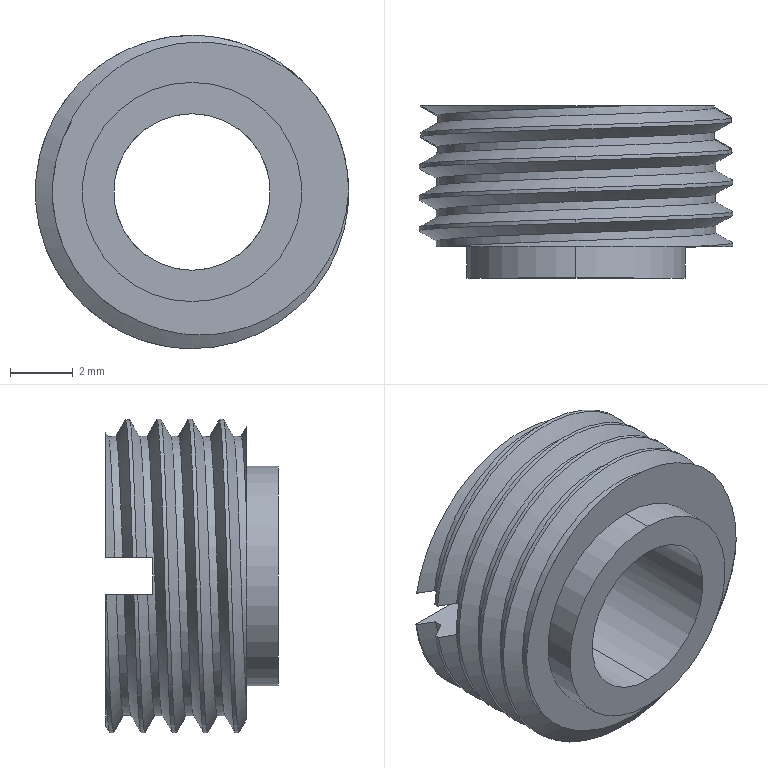Part | STEP file | 1 solid | 38 faces | box 10 x 5.5 x 10 mm | volume 234.976 mm3 | cylinder 20 | plane 10 | spline 8 | commonest cylinder face diameters 10 x12 8.917 x4 5 x2 7 x2